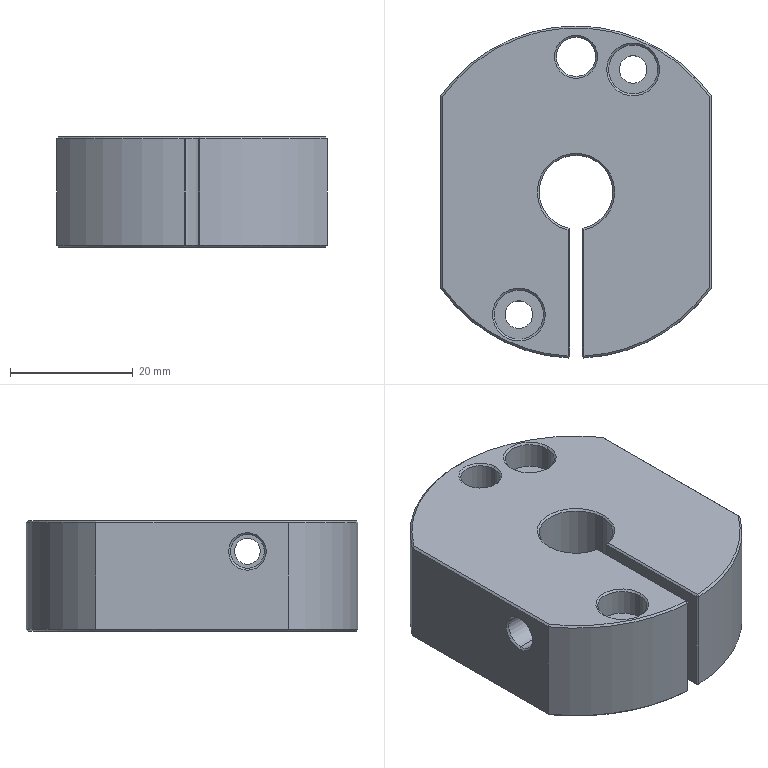Part | SolidWorks | features ICE 4, HoleWzd 2, Chamfer 1, CirPattern 1, Extrusion 1 | 1 solid | 70 faces | box 44 x 53.969 x 18 mm | volume 32312 mm3 | cone 28 | plane 22 | cylinder 20 | commonest cylinder face diameters 4.5 x4 8 x4 12 x3 54 x3 4.2 x2 5.5 x2